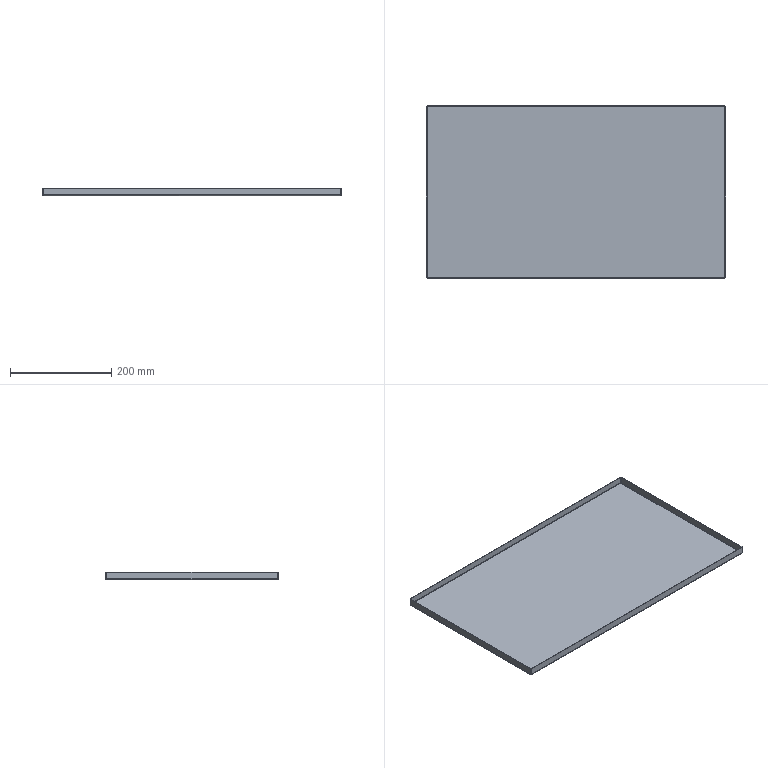Part | NX | features BREP 1 | 1 solid | 38 faces | box 590 x 340 x 15 mm | volume 336698 mm3 | plane 22 | spline 8 | cylinder 8 | commonest cylinder face diameters 1 x4 4 x4
STEP:
#1=CARTESIAN_POINT('',(293.,-168.,-1.5));
#2=VERTEX_POINT('',#1);
#3=CARTESIAN_POINT('',(-293.,-168.,-1.5));
#4=VERTEX_POINT('',#3);
#5=CARTESIAN_POINT('',(293.,-168.,-1.5));
#6=DIRECTION('',(-1.,0.,0.));
#7=VECTOR('',#6,1000.);
#8=LINE('',#5,#7);
#9=EDGE_CURVE('',#2,#4,#8,.T.);
#10=ORIENTED_EDGE('',*,*,#9,.T.);
#11=CARTESIAN_POINT('',(-293.,168.,-1.5));
#12=VERTEX_POINT('',#11);
#13=CARTESIAN_POINT('',(-293.,-168.,-1.5));
#14=DIRECTION('',(0.,1.,0.));
#15=VECTOR('',#14,1000.);
#16=LINE('',#13,#15);
#17=EDGE_CURVE('',#4,#12,#16,.T.);
#18=ORIENTED_EDGE('',*,*,#17,.T.);
#19=CARTESIAN_POINT('',(293.,168.,-1.5));
#20=VERTEX_POINT('',#19);
#21=CARTESIAN_POINT('',(-293.,168.,-1.5));
#22=DIRECTION('',(1.,0.,0.));
#23=VECTOR('',#22,1000.);
#24=LINE('',#21,#23);
#25=EDGE_CURVE('',#12,#20,#24,.T.);
#26=ORIENTED_EDGE('',*,*,#25,.T.);
#27=CARTESIAN_POINT('',(293.,168.,-1.5));
#28=DIRECTION('',(0.,-1.,0.));
#29=VECTOR('',#28,1000.);
#30=LINE('',#27,#29);
#31=EDGE_CURVE('',#20,#2,#30,.T.);
#32=ORIENTED_EDGE('',*,*,#31,.T.);
#33=EDGE_LOOP('',(#10,#18,#26,#32));
#34=FACE_BOUND('',#33,.T.);
#35=CARTESIAN_POINT('',(0.,0.,-1.5));
#36=DIRECTION('',(0.,0.,-1.));
#37=DIRECTION('',(0.,-1.,0.));
#38=AXIS2_PLACEMENT_3D('',#35,#36,#37);
#39=PLANE('',#38);
#40=ADVANCED_FACE('',(#34),#39,.T.);
#41=CARTESIAN_POINT('',(-293.,-168.,0.));
#42=VERTEX_POINT('',#41);
#43=CARTESIAN_POINT('',(-293.,168.,0.));
#44=VERTEX_POINT('',#43);
#45=CARTESIAN_POINT('',(-293.,-168.,0.));
#46=DIRECTION('',(0.,1.,0.));
#47=VECTOR('',#46,1000.);
#48=LINE('',#45,#47);
#49=EDGE_CURVE('',#42,#44,#48,.T.);
#50=ORIENTED_EDGE('',*,*,#49,.F.);
#51=CARTESIAN_POINT('',(293.,-168.,0.));
#52=VERTEX_POINT('',#51);
#53=CARTESIAN_POINT('',(293.,-168.,0.));
#54=DIRECTION('',(-1.,0.,0.));
#55=VECTOR('',#54,1000.);
#56=LINE('',#53,#55);
#57=EDGE_CURVE('',#52,#42,#56,.T.);
#58=ORIENTED_EDGE('',*,*,#57,.F.);
#59=CARTESIAN_POINT('',(293.,168.,0.));
#60=VERTEX_POINT('',#59);
#61=CARTESIAN_POINT('',(293.,168.,0.));
#62=DIRECTION('',(0.,-1.,0.));
#63=VECTOR('',#62,1000.);
#64=LINE('',#61,#63);
#65=EDGE_CURVE('',#60,#52,#64,.T.);
#66=ORIENTED_EDGE('',*,*,#65,.F.);
#67=CARTESIAN_POINT('',(-293.,168.,0.));
#68=DIRECTION('',(1.,0.,0.));
#69=VECTOR('',#68,1000.);
#70=LINE('',#67,#69);
#71=EDGE_CURVE('',#44,#60,#70,.T.);
#72=ORIENTED_EDGE('',*,*,#71,.F.);
#73=EDGE_LOOP('',(#50,#58,#66,#72));
#74=FACE_BOUND('',#73,.T.);
#75=CARTESIAN_POINT('',(0.,0.,0.));
#76=DIRECTION('',(0.,0.,-1.));
#77=DIRECTION('',(0.,-1.,0.));
#78=AXIS2_PLACEMENT_3D('',#75,#76,#77);
#79=PLANE('',#78);
#80=ADVANCED_FACE('',(#74),#79,.F.);
#81=CARTESIAN_POINT('',(292.793,170.,0.5));
#82=VERTEX_POINT('',#81);
#83=CARTESIAN_POINT('',(292.793,168.5,0.5));
#84=VERTEX_POINT('',#83);
#85=CARTESIAN_POINT('',(292.793,168.5,0.5));
#86=DIRECTION('',(0.,-1.,0.));
#87=VECTOR('',#86,1000.);
#88=LINE('',#85,#87);
#89=EDGE_CURVE('',#82,#84,#88,.T.);
#90=ORIENTED_EDGE('',*,*,#89,.T.);
#91=CARTESIAN_POINT('',(293.,168.,0.));
#92=CARTESIAN_POINT('',(292.931,168.262,0.));
#93=CARTESIAN_POINT('',(292.862,168.5,0.2382));
#94=CARTESIAN_POINT('',(292.793,168.5,0.5));
#95=B_SPLINE_CURVE_WITH_KNOTS('',3,(#91,#92,#93,#94),.UNSPECIFIED.,.F.,.F.,(4,4),(0.,1.),.UNSPECIFIED.);
#96=EDGE_CURVE('',#60,#84,#95,.T.);
#97=ORIENTED_EDGE('',*,*,#96,.F.);
#98=CARTESIAN_POINT('',(293.,168.,0.));
#99=DIRECTION('',(0.,0.,-1.));
#100=VECTOR('',#99,1000.);
#101=LINE('',#98,#100);
#102=EDGE_CURVE('',#60,#20,#101,.T.);
#103=ORIENTED_EDGE('',*,*,#102,.T.);
#104=CARTESIAN_POINT('',(292.793,170.,0.5));
#105=CARTESIAN_POINT('',(292.827,170.,-0.0236));
#106=CARTESIAN_POINT('',(292.896,169.567,-1.067));
#107=CARTESIAN_POINT('',(292.965,168.524,-1.5));
#108=CARTESIAN_POINT('',(293.,168.,-1.5));
#109=B_SPLINE_CURVE_WITH_KNOTS('',3,(#104,#105,#106,#107,#108),.UNSPECIFIED.,.F.,.F.,(4,1,4),(0.,0.5,1.),.UNSPECIFIED.);
#110=EDGE_CURVE('',#20,#82,#109,.F.);
#111=ORIENTED_EDGE('',*,*,#110,.T.);
#112=EDGE_LOOP('',(#90,#97,#103,#111));
#113=FACE_BOUND('',#112,.T.);
#114=CARTESIAN_POINT('',(293.,168.,-1.515));
#115=CARTESIAN_POINT('',(292.983,168.264,-1.515));
#116=CARTESIAN_POINT('',(292.965,168.527,-1.463));
#117=CARTESIAN_POINT('',(292.931,169.015,-1.261));
#118=CARTESIAN_POINT('',(292.914,169.238,-1.111));
#119=CARTESIAN_POINT('',(292.879,169.611,-0.7383));
#120=CARTESIAN_POINT('',(292.862,169.761,-0.5148));
#121=CARTESIAN_POINT('',(292.827,169.963,-0.02742));
#122=CARTESIAN_POINT('',(292.81,170.015,0.2362));
#123=CARTESIAN_POINT('',(292.793,170.015,0.5));
#124=CARTESIAN_POINT('',(293.,168.,-1.5));
#125=CARTESIAN_POINT('',(292.983,168.262,-1.5));
#126=CARTESIAN_POINT('',(292.965,168.523,-1.448));
#127=CARTESIAN_POINT('',(292.931,169.007,-1.248));
#128=CARTESIAN_POINT('',(292.914,169.229,-1.099));
#129=CARTESIAN_POINT('',(292.879,169.599,-0.7291));
#130=CARTESIAN_POINT('',(292.862,169.748,-0.5072));
#131=CARTESIAN_POINT('',(292.827,169.948,-0.0235));
#132=CARTESIAN_POINT('',(292.81,170.,0.2382));
#133=CARTESIAN_POINT('',(292.793,170.,0.5));
#134=CARTESIAN_POINT('',(293.,168.,0.));
#135=CARTESIAN_POINT('',(292.983,168.065,0.));
#136=CARTESIAN_POINT('',(292.965,168.131,0.01301));
#137=CARTESIAN_POINT('',(292.931,168.252,0.06311));
#138=CARTESIAN_POINT('',(292.914,168.307,0.1002));
#139=CARTESIAN_POINT('',(292.879,168.4,0.1927));
#140=CARTESIAN_POINT('',(292.862,168.437,0.2482));
#141=CARTESIAN_POINT('',(292.827,168.487,0.3691));
#142=CARTESIAN_POINT('',(292.81,168.5,0.4345));
#143=CARTESIAN_POINT('',(292.793,168.5,0.5));
#144=CARTESIAN_POINT('',(293.,168.,0.01515));
#145=CARTESIAN_POINT('',(292.983,168.063,0.01515));
#146=CARTESIAN_POINT('',(292.965,168.127,0.02777));
#147=CARTESIAN_POINT('',(292.931,168.244,0.07634));
#148=CARTESIAN_POINT('',(292.914,168.298,0.1123));
#149=CARTESIAN_POINT('',(292.879,168.388,0.202));
#150=CARTESIAN_POINT('',(292.862,168.424,0.2558));
#151=CARTESIAN_POINT('',(292.827,168.472,0.3731));
#152=CARTESIAN_POINT('',(292.81,168.485,0.4365));
#153=CARTESIAN_POINT('',(292.793,168.485,0.5));
#154=B_SPLINE_SURFACE_WITH_KNOTS('',1,3,((#114,#115,#116,#117,#118,#119,#120,#121,#122,#123),(#124,#125,#126,#127,#128,#129,#130,#131,#132,#133),(#134,#135,#136,#137,#138,#139,#140,#141,#142,#143),(#144,#145,#146,#147,#148,#149,#150,#151,#152,#153)),.RULED_SURF.,.F.,.F.,.F.,(2,1,1,2),(4,2,2,2,4),(-0.01,0.,1.,1.01),(0.,0.25,0.5,0.75,1.),.UNSPECIFIED.);
#155=ADVANCED_FACE('',(#113),#154,.F.);
#156=CARTESIAN_POINT('',(-292.793,168.5,0.5));
#157=VERTEX_POINT('',#156);
#158=CARTESIAN_POINT('',(-292.793,168.5,0.5));
#159=CARTESIAN_POINT('',(-292.862,168.5,0.2382));
#160=CARTESIAN_POINT('',(-292.931,168.262,0.));
#161=CARTESIAN_POINT('',(-293.,168.,0.));
#162=B_SPLINE_CURVE_WITH_KNOTS('',3,(#158,#159,#160,#161),.UNSPECIFIED.,.F.,.F.,(4,4),(0.,1.),.UNSPECIFIED.);
#163=EDGE_CURVE('',#157,#44,#162,.T.);
#164=ORIENTED_EDGE('',*,*,#163,.F.);
#165=CARTESIAN_POINT('',(-292.793,170.,0.5));
#166=VERTEX_POINT('',#165);
#167=CARTESIAN_POINT('',(-292.793,168.5,0.5));
#168=DIRECTION('',(0.,-1.,0.));
#169=VECTOR('',#168,1000.);
#170=LINE('',#167,#169);
#171=EDGE_CURVE('',#166,#157,#170,.T.);
#172=ORIENTED_EDGE('',*,*,#171,.F.);
#173=CARTESIAN_POINT('',(-293.,168.,-1.5));
#174=CARTESIAN_POINT('',(-292.965,168.524,-1.5));
#175=CARTESIAN_POINT('',(-292.896,169.567,-1.067));
#176=CARTESIAN_POINT('',(-292.827,170.,-0.0236));
#177=CARTESIAN_POINT('',(-292.793,170.,0.5));
#178=B_SPLINE_CURVE_WITH_KNOTS('',3,(#173,#174,#175,#176,#177),.UNSPECIFIED.,.F.,.F.,(4,1,4),(0.,0.5,1.),.UNSPECIFIED.);
#179=EDGE_CURVE('',#166,#12,#178,.F.);
#180=ORIENTED_EDGE('',*,*,#179,.T.);
#181=CARTESIAN_POINT('',(-293.,168.,0.));
#182=DIRECTION('',(0.,0.,-1.));
#183=VECTOR('',#182,1000.);
#184=LINE('',#181,#183);
#185=EDGE_CURVE('',#44,#12,#184,.T.);
#186=ORIENTED_EDGE('',*,*,#185,.F.);
#187=EDGE_LOOP('',(#164,#172,#180,#186));
#188=FACE_BOUND('',#187,.T.);
#189=CARTESIAN_POINT('',(-292.793,170.015,0.5));
#190=CARTESIAN_POINT('',(-292.81,170.015,0.2362));
#191=CARTESIAN_POINT('',(-292.827,169.963,-0.02742));
#192=CARTESIAN_POINT('',(-292.862,169.761,-0.5148));
#193=CARTESIAN_POINT('',(-292.879,169.611,-0.7383));
#194=CARTESIAN_POINT('',(-292.914,169.238,-1.111));
#195=CARTESIAN_POINT('',(-292.931,169.015,-1.261));
#196=CARTESIAN_POINT('',(-292.965,168.527,-1.463));
#197=CARTESIAN_POINT('',(-292.983,168.264,-1.515));
#198=CARTESIAN_POINT('',(-293.,168.,-1.515));
#199=CARTESIAN_POINT('',(-292.793,170.,0.5));
#200=CARTESIAN_POINT('',(-292.81,170.,0.2382));
#201=CARTESIAN_POINT('',(-292.827,169.948,-0.0235));
#202=CARTESIAN_POINT('',(-292.862,169.748,-0.5072));
#203=CARTESIAN_POINT('',(-292.879,169.599,-0.7291));
#204=CARTESIAN_POINT('',(-292.914,169.229,-1.099));
#205=CARTESIAN_POINT('',(-292.931,169.007,-1.248));
#206=CARTESIAN_POINT('',(-292.965,168.523,-1.448));
#207=CARTESIAN_POINT('',(-292.983,168.262,-1.5));
#208=CARTESIAN_POINT('',(-293.,168.,-1.5));
#209=CARTESIAN_POINT('',(-292.793,168.5,0.5));
#210=CARTESIAN_POINT('',(-292.81,168.5,0.4345));
#211=CARTESIAN_POINT('',(-292.827,168.487,0.3691));
#212=CARTESIAN_POINT('',(-292.862,168.437,0.2482));
#213=CARTESIAN_POINT('',(-292.879,168.4,0.1927));
#214=CARTESIAN_POINT('',(-292.914,168.307,0.1002));
#215=CARTESIAN_POINT('',(-292.931,168.252,0.06311));
#216=CARTESIAN_POINT('',(-292.965,168.131,0.01301));
#217=CARTESIAN_POINT('',(-292.983,168.065,0.));
#218=CARTESIAN_POINT('',(-293.,168.,0.));
#219=CARTESIAN_POINT('',(-292.793,168.485,0.5));
#220=CARTESIAN_POINT('',(-292.81,168.485,0.4365));
#221=CARTESIAN_POINT('',(-292.827,168.472,0.3731));
#222=CARTESIAN_POINT('',(-292.862,168.424,0.2558));
#223=CARTESIAN_POINT('',(-292.879,168.388,0.202));
#224=CARTESIAN_POINT('',(-292.914,168.298,0.1123));
#225=CARTESIAN_POINT('',(-292.931,168.244,0.07634));
#226=CARTESIAN_POINT('',(-292.965,168.127,0.02777));
#227=CARTESIAN_POINT('',(-292.983,168.063,0.01515));
#228=CARTESIAN_POINT('',(-293.,168.,0.01515));
#229=B_SPLINE_SURFACE_WITH_KNOTS('',1,3,((#189,#190,#191,#192,#193,#194,#195,#196,#197,#198),(#199,#200,#201,#202,#203,#204,#205,#206,#207,#208),(#209,#210,#211,#212,#213,#214,#215,#216,#217,#218),(#219,#220,#221,#222,#223,#224,#225,#226,#227,#228)),.RULED_SURF.,.F.,.F.,.F.,(2,1,1,2),(4,2,2,2,4),(-0.01,0.,1.,1.01),(0.,0.25,0.5,0.75,1.),.UNSPECIFIED.);
#230=ADVANCED_FACE('',(#188),#229,.F.);
#231=ORIENTED_EDGE('',*,*,#25,.F.);
#232=ORIENTED_EDGE('',*,*,#179,.F.);
#233=CARTESIAN_POINT('',(0.,170.,0.5));
#234=DIRECTION('',(-1.,0.,0.));
#235=VECTOR('',#234,1000.);
#236=LINE('',#233,#235);
#237=EDGE_CURVE('',#82,#166,#236,.T.);
#238=ORIENTED_EDGE('',*,*,#237,.F.);
#239=ORIENTED_EDGE('',*,*,#110,.F.);
#240=EDGE_LOOP('',(#231,#232,#238,#239));
#241=FACE_BOUND('',#240,.T.);
#242=CARTESIAN_POINT('',(-293.,168.,0.5));
#243=DIRECTION('',(-1.,0.,0.));
#244=DIRECTION('',(0.,1.,0.));
#245=AXIS2_PLACEMENT_3D('',#242,#243,#244);
#246=CYLINDRICAL_SURFACE('',#245,2.);
#247=ADVANCED_FACE('',(#241),#246,.T.);
#248=ORIENTED_EDGE('',*,*,#71,.T.);
#249=ORIENTED_EDGE('',*,*,#96,.T.);
#250=CARTESIAN_POINT('',(295.,168.5,0.5));
#251=DIRECTION('',(-1.,0.,0.));
#252=VECTOR('',#251,1000.);
#253=LINE('',#250,#252);
#254=EDGE_CURVE('',#84,#157,#253,.T.);
#255=ORIENTED_EDGE('',*,*,#254,.T.);
#256=ORIENTED_EDGE('',*,*,#163,.T.);
#257=EDGE_LOOP('',(#248,#249,#255,#256));
#258=FACE_BOUND('',#257,.T.);
#259=CARTESIAN_POINT('',(-293.,168.,0.5));
#260=DIRECTION('',(-1.,0.,0.));
#261=DIRECTION('',(0.,1.,0.));
#262=AXIS2_PLACEMENT_3D('',#259,#260,#261);
#263=CYLINDRICAL_SURFACE('',#262,0.5);
#264=ADVANCED_FACE('',(#258),#263,.F.);
#265=CARTESIAN_POINT('',(292.793,168.5,13.5));
#266=VERTEX_POINT('',#265);
#267=CARTESIAN_POINT('',(292.793,170.,13.5));
#268=VERTEX_POINT('',#267);
#269=CARTESIAN_POINT('',(292.793,170.,13.5));
#270=DIRECTION('',(0.,1.,0.));
#271=VECTOR('',#270,1000.);
#272=LINE('',#269,#271);
#273=EDGE_CURVE('',#266,#268,#272,.T.);
#274=ORIENTED_EDGE('',*,*,#273,.F.);
#275=CARTESIAN_POINT('',(292.793,168.5,0.));
#276=DIRECTION('',(0.,0.,1.));
#277=VECTOR('',#276,1000.);
#278=LINE('',#275,#277);
#279=EDGE_CURVE('',#84,#266,#278,.T.);
#280=ORIENTED_EDGE('',*,*,#279,.F.);
#281=ORIENTED_EDGE('',*,*,#89,.F.);
#282=CARTESIAN_POINT('',(292.793,170.,0.));
#283=DIRECTION('',(0.,0.,-1.));
#284=VECTOR('',#283,1000.);
#285=LINE('',#282,#284);
#286=EDGE_CURVE('',#268,#82,#285,.T.);
#287=ORIENTED_EDGE('',*,*,#286,.F.);
#288=EDGE_LOOP('',(#274,#280,#281,#287));
#289=FACE_BOUND('',#288,.T.);
#290=CARTESIAN_POINT('',(292.793,168.5,0.));
#291=DIRECTION('',(1.,0.,0.));
#292=DIRECTION('',(0.,1.,0.));
#293=AXIS2_PLACEMENT_3D('',#290,#291,#292);
#294=PLANE('',#293);
#295=ADVANCED_FACE('',(#289),#294,.T.);
#296=CARTESIAN_POINT('',(-292.793,170.,13.5));
#297=VERTEX_POINT('',#296);
#298=CARTESIAN_POINT('',(-292.793,170.,0.));
#299=DIRECTION('',(0.,0.,-1.));
#300=VECTOR('',#299,1000.);
#301=LINE('',#298,#300);
#302=EDGE_CURVE('',#297,#166,#301,.T.);
#303=ORIENTED_EDGE('',*,*,#302,.F.);
#304=CARTESIAN_POINT('',(-295.,170.,13.5));
#305=DIRECTION('',(-1.,0.,0.));
#306=VECTOR('',#305,1000.);
#307=LINE('',#304,#306);
#308=EDGE_CURVE('',#268,#297,#307,.T.);
#309=ORIENTED_EDGE('',*,*,#308,.F.);
#310=ORIENTED_EDGE('',*,*,#286,.T.);
#311=ORIENTED_EDGE('',*,*,#237,.T.);
#312=EDGE_LOOP('',(#303,#309,#310,#311));
#313=FACE_BOUND('',#312,.T.);
#314=CARTESIAN_POINT('',(0.,170.,0.));
#315=DIRECTION('',(0.,1.,0.));
#316=DIRECTION('',(0.,0.,-1.));
#317=AXIS2_PLACEMENT_3D('',#314,#315,#316);
#318=PLANE('',#317);
#319=ADVANCED_FACE('',(#313),#318,.T.);
#320=CARTESIAN_POINT('',(-292.793,168.5,13.5));
#321=VERTEX_POINT('',#320);
#322=CARTESIAN_POINT('',(0.,168.5,13.5));
#323=DIRECTION('',(-1.,0.,0.));
#324=VECTOR('',#323,1000.);
#325=LINE('',#322,#324);
#326=EDGE_CURVE('',#266,#321,#325,.T.);
#327=ORIENTED_EDGE('',*,*,#326,.T.);
#328=CARTESIAN_POINT('',(-292.793,168.5,0.));
#329=DIRECTION('',(0.,0.,1.));
#330=VECTOR('',#329,1000.);
#331=LINE('',#328,#330);
#332=EDGE_CURVE('',#157,#321,#331,.T.);
#333=ORIENTED_EDGE('',*,*,#332,.F.);
#334=ORIENTED_EDGE('',*,*,#254,.F.);
#335=ORIENTED_EDGE('',*,*,#279,.T.);
#336=EDGE_LOOP('',(#327,#333,#334,#335));
#337=FACE_BOUND('',#336,.T.);
#338=CARTESIAN_POINT('',(0.,168.5,0.));
#339=DIRECTION('',(0.,1.,0.));
#340=DIRECTION('',(0.,0.,-1.));
#341=AXIS2_PLACEMENT_3D('',#338,#339,#340);
#342=PLANE('',#341);
#343=ADVANCED_FACE('',(#337),#342,.F.);
#344=CARTESIAN_POINT('',(-292.793,168.5,13.5));
#345=DIRECTION('',(0.,1.,0.));
#346=VECTOR('',#345,1000.);
#347=LINE('',#344,#346);
#348=EDGE_CURVE('',#321,#297,#347,.T.);
#349=ORIENTED_EDGE('',*,*,#348,.F.);
#350=ORIENTED_EDGE('',*,*,#326,.F.);
#351=ORIENTED_EDGE('',*,*,#273,.T.);
#352=ORIENTED_EDGE('',*,*,#308,.T.);
#353=EDGE_LOOP('',(#349,#350,#351,#352));
#354=FACE_BOUND('',#353,.T.);
#355=CARTESIAN_POINT('',(-295.,170.,13.5));
#356=DIRECTION('',(0.,0.,1.));
#357=DIRECTION('',(0.,-1.,0.));
#358=AXIS2_PLACEMENT_3D('',#355,#356,#357);
#359=PLANE('',#358);
#360=ADVANCED_FACE('',(#354),#359,.T.);
#361=ORIENTED_EDGE('',*,*,#332,.T.);
#362=ORIENTED_EDGE('',*,*,#348,.T.);
#363=ORIENTED_EDGE('',*,*,#302,.T.);
#364=ORIENTED_EDGE('',*,*,#171,.T.);
#365=EDGE_LOOP('',(#361,#362,#363,#364));
#366=FACE_BOUND('',#365,.T.);
#367=CARTESIAN_POINT('',(-292.793,168.5,0.));
#368=DIRECTION('',(1.,0.,0.));
#369=DIRECTION('',(0.,1.,0.));
#370=AXIS2_PLACEMENT_3D('',#367,#368,#369);
#371=PLANE('',#370);
#372=ADVANCED_FACE('',(#366),#371,.F.);
#373=CARTESIAN_POINT('',(295.,-167.793,0.5));
#374=VERTEX_POINT('',#373);
#375=CARTESIAN_POINT('',(293.5,-167.793,0.5));
#376=VERTEX_POINT('',#375);
#377=CARTESIAN_POINT('',(293.5,-167.793,0.5));
#378=DIRECTION('',(-1.,0.,0.));
#379=VECTOR('',#378,1000.);
#380=LINE('',#377,#379);
#381=EDGE_CURVE('',#374,#376,#380,.T.);
#382=ORIENTED_EDGE('',*,*,#381,.T.);
#383=CARTESIAN_POINT('',(293.,-168.,0.));
#384=CARTESIAN_POINT('',(293.262,-167.931,0.));
#385=CARTESIAN_POINT('',(293.5,-167.862,0.2382));
#386=CARTESIAN_POINT('',(293.5,-167.793,0.5));
#387=B_SPLINE_CURVE_WITH_KNOTS('',3,(#383,#384,#385,#386),.UNSPECIFIED.,.F.,.F.,(4,4),(0.,1.),.UNSPECIFIED.);
#388=EDGE_CURVE('',#52,#376,#387,.T.);
#389=ORIENTED_EDGE('',*,*,#388,.F.);
#390=CARTESIAN_POINT('',(293.,-168.,0.));
#391=DIRECTION('',(0.,0.,-1.));
#392=VECTOR('',#391,1000.);
#393=LINE('',#390,#392);
#394=EDGE_CURVE('',#52,#2,#393,.T.);
#395=ORIENTED_EDGE('',*,*,#394,.T.);
#396=CARTESIAN_POINT('',(295.,-167.793,0.5));
#397=CARTESIAN_POINT('',(295.,-167.827,-0.0236));
#398=CARTESIAN_POINT('',(294.567,-167.896,-1.067));
#399=CARTESIAN_POINT('',(293.524,-167.965,-1.5));
#400=CARTESIAN_POINT('',(293.,-168.,-1.5));
#401=B_SPLINE_CURVE_WITH_KNOTS('',3,(#396,#397,#398,#399,#400),.UNSPECIFIED.,.F.,.F.,(4,1,4),(0.,0.5,1.),.UNSPECIFIED.);
#402=EDGE_CURVE('',#2,#374,#401,.F.);
#403=ORIENTED_EDGE('',*,*,#402,.T.);
#404=EDGE_LOOP('',(#382,#389,#395,#403));
#405=FACE_BOUND('',#404,.T.);
#406=CARTESIAN_POINT('',(293.,-168.,-1.515));
#407=CARTESIAN_POINT('',(293.264,-167.983,-1.515));
#408=CARTESIAN_POINT('',(293.527,-167.965,-1.463));
#409=CARTESIAN_POINT('',(294.015,-167.931,-1.261));
#410=CARTESIAN_POINT('',(294.238,-167.914,-1.111));
#411=CARTESIAN_POINT('',(294.611,-167.879,-0.7383));
#412=CARTESIAN_POINT('',(294.761,-167.862,-0.5148));
#413=CARTESIAN_POINT('',(294.963,-167.827,-0.02742));
#414=CARTESIAN_POINT('',(295.015,-167.81,0.2362));
#415=CARTESIAN_POINT('',(295.015,-167.793,0.5));
#416=CARTESIAN_POINT('',(293.,-168.,-1.5));
#417=CARTESIAN_POINT('',(293.262,-167.983,-1.5));
#418=CARTESIAN_POINT('',(293.523,-167.965,-1.448));
#419=CARTESIAN_POINT('',(294.007,-167.931,-1.248));
#420=CARTESIAN_POINT('',(294.229,-167.914,-1.099));
#421=CARTESIAN_POINT('',(294.599,-167.879,-0.7291));
#422=CARTESIAN_POINT('',(294.748,-167.862,-0.5072));
#423=CARTESIAN_POINT('',(294.948,-167.827,-0.0235));
#424=CARTESIAN_POINT('',(295.,-167.81,0.2382));
#425=CARTESIAN_POINT('',(295.,-167.793,0.5));
#426=CARTESIAN_POINT('',(293.,-168.,0.));
#427=CARTESIAN_POINT('',(293.065,-167.983,0.));
#428=CARTESIAN_POINT('',(293.131,-167.965,0.01301));
#429=CARTESIAN_POINT('',(293.252,-167.931,0.06311));
#430=CARTESIAN_POINT('',(293.307,-167.914,0.1002));
#431=CARTESIAN_POINT('',(293.4,-167.879,0.1927));
#432=CARTESIAN_POINT('',(293.437,-167.862,0.2482));
#433=CARTESIAN_POINT('',(293.487,-167.827,0.3691));
#434=CARTESIAN_POINT('',(293.5,-167.81,0.4345));
#435=CARTESIAN_POINT('',(293.5,-167.793,0.5));
#436=CARTESIAN_POINT('',(293.,-168.,0.01515));
#437=CARTESIAN_POINT('',(293.063,-167.983,0.01515));
#438=CARTESIAN_POINT('',(293.127,-167.965,0.02777));
#439=CARTESIAN_POINT('',(293.244,-167.931,0.07634));
#440=CARTESIAN_POINT('',(293.298,-167.914,0.1123));
#441=CARTESIAN_POINT('',(293.388,-167.879,0.202));
#442=CARTESIAN_POINT('',(293.424,-167.862,0.2558));
#443=CARTESIAN_POINT('',(293.472,-167.827,0.3731));
#444=CARTESIAN_POINT('',(293.485,-167.81,0.4365));
#445=CARTESIAN_POINT('',(293.485,-167.793,0.5));
#446=B_SPLINE_SURFACE_WITH_KNOTS('',1,3,((#406,#407,#408,#409,#410,#411,#412,#413,#414,#415),(#416,#417,#418,#419,#420,#421,#422,#423,#424,#425),(#426,#427,#428,#429,#430,#431,#432,#433,#434,#435),(#436,#437,#438,#439,#440,#441,#442,#443,#444,#445)),.RULED_SURF.,.F.,.F.,.F.,(2,1,1,2),(4,2,2,2,4),(-0.01,0.,1.,1.01),(0.,0.25,0.5,0.75,1.),.UNSPECIFIED.);
#447=ADVANCED_FACE('',(#405),#446,.F.);
#448=CARTESIAN_POINT('',(293.5,167.793,0.5));
#449=VERTEX_POINT('',#448);
#450=CARTESIAN_POINT('',(293.5,167.793,0.5));
#451=CARTESIAN_POINT('',(293.5,167.862,0.2382));
#452=CARTESIAN_POINT('',(293.262,167.931,0.));
#453=CARTESIAN_POINT('',(293.,168.,0.));
#454=B_SPLINE_CURVE_WITH_KNOTS('',3,(#450,#451,#452,#453),.UNSPECIFIED.,.F.,.F.,(4,4),(0.,1.),.UNSPECIFIED.);
#455=EDGE_CURVE('',#449,#60,#454,.T.);
#456=ORIENTED_EDGE('',*,*,#455,.F.);
#457=CARTESIAN_POINT('',(295.,167.793,0.5));
#458=VERTEX_POINT('',#457);
#459=CARTESIAN_POINT('',(293.5,167.793,0.5));
#460=DIRECTION('',(-1.,0.,0.));
#461=VECTOR('',#460,1000.);
#462=LINE('',#459,#461);
#463=EDGE_CURVE('',#458,#449,#462,.T.);
#464=ORIENTED_EDGE('',*,*,#463,.F.);
#465=CARTESIAN_POINT('',(293.,168.,-1.5));
#466=CARTESIAN_POINT('',(293.524,167.965,-1.5));
#467=CARTESIAN_POINT('',(294.567,167.896,-1.067));
#468=CARTESIAN_POINT('',(295.,167.827,-0.0236));
#469=CARTESIAN_POINT('',(295.,167.793,0.5));
#470=B_SPLINE_CURVE_WITH_KNOTS('',3,(#465,#466,#467,#468,#469),.UNSPECIFIED.,.F.,.F.,(4,1,4),(0.,0.5,1.),.UNSPECIFIED.);
#471=EDGE_CURVE('',#458,#20,#470,.F.);
#472=ORIENTED_EDGE('',*,*,#471,.T.);
#473=ORIENTED_EDGE('',*,*,#102,.F.);
#474=EDGE_LOOP('',(#456,#464,#472,#473));
#475=FACE_BOUND('',#474,.T.);
#476=CARTESIAN_POINT('',(295.015,167.793,0.5));
#477=CARTESIAN_POINT('',(295.015,167.81,0.2362));
#478=CARTESIAN_POINT('',(294.963,167.827,-0.02742));
#479=CARTESIAN_POINT('',(294.761,167.862,-0.5148));
#480=CARTESIAN_POINT('',(294.611,167.879,-0.7383));
#481=CARTESIAN_POINT('',(294.238,167.914,-1.111));
#482=CARTESIAN_POINT('',(294.015,167.931,-1.261));
#483=CARTESIAN_POINT('',(293.527,167.965,-1.463));
#484=CARTESIAN_POINT('',(293.264,167.983,-1.515));
#485=CARTESIAN_POINT('',(293.,168.,-1.515));
#486=CARTESIAN_POINT('',(295.,167.793,0.5));
#487=CARTESIAN_POINT('',(295.,167.81,0.2382));
#488=CARTESIAN_POINT('',(294.948,167.827,-0.0235));
#489=CARTESIAN_POINT('',(294.748,167.862,-0.5072));
#490=CARTESIAN_POINT('',(294.599,167.879,-0.7291));
#491=CARTESIAN_POINT('',(294.229,167.914,-1.099));
#492=CARTESIAN_POINT('',(294.007,167.931,-1.248));
#493=CARTESIAN_POINT('',(293.523,167.965,-1.448));
#494=CARTESIAN_POINT('',(293.262,167.983,-1.5));
#495=CARTESIAN_POINT('',(293.,168.,-1.5));
#496=CARTESIAN_POINT('',(293.5,167.793,0.5));
#497=CARTESIAN_POINT('',(293.5,167.81,0.4345));
#498=CARTESIAN_POINT('',(293.487,167.827,0.3691));
#499=CARTESIAN_POINT('',(293.437,167.862,0.2482));
#500=CARTESIAN_POINT('',(293.4,167.879,0.1927));
#501=CARTESIAN_POINT('',(293.307,167.914,0.1002));
#502=CARTESIAN_POINT('',(293.252,167.931,0.06311));
#503=CARTESIAN_POINT('',(293.131,167.965,0.01301));
#504=CARTESIAN_POINT('',(293.065,167.983,0.));
#505=CARTESIAN_POINT('',(293.,168.,0.));
#506=CARTESIAN_POINT('',(293.485,167.793,0.5));
#507=CARTESIAN_POINT('',(293.485,167.81,0.4365));
#508=CARTESIAN_POINT('',(293.472,167.827,0.3731));
#509=CARTESIAN_POINT('',(293.424,167.862,0.2558));
#510=CARTESIAN_POINT('',(293.388,167.879,0.202));
#511=CARTESIAN_POINT('',(293.298,167.914,0.1123));
#512=CARTESIAN_POINT('',(293.244,167.931,0.07634));
#513=CARTESIAN_POINT('',(293.127,167.965,0.02777));
#514=CARTESIAN_POINT('',(293.063,167.983,0.01515));
#515=CARTESIAN_POINT('',(293.,168.,0.01515));
#516=B_SPLINE_SURFACE_WITH_KNOTS('',1,3,((#476,#477,#478,#479,#480,#481,#482,#483,#484,#485),(#486,#487,#488,#489,#490,#491,#492,#493,#494,#495),(#496,#497,#498,#499,#500,#501,#502,#503,#504,#505),(#506,#507,#508,#509,#510,#511,#512,#513,#514,#515)),.RULED_SURF.,.F.,.F.,.F.,(2,1,1,2),(4,2,2,2,4),(-0.01,0.,1.,1.01),(0.,0.25,0.5,0.75,1.),.UNSPECIFIED.);
#517=ADVANCED_FACE('',(#475),#516,.F.);
#518=ORIENTED_EDGE('',*,*,#31,.F.);
#519=ORIENTED_EDGE('',*,*,#471,.F.);
#520=CARTESIAN_POINT('',(295.,-170.,0.5));
#521=DIRECTION('',(0.,-1.,0.));
#522=VECTOR('',#521,1000.);
#523=LINE('',#520,#522);
#524=EDGE_CURVE('',#458,#374,#523,.T.);
#525=ORIENTED_EDGE('',*,*,#524,.T.);
#526=ORIENTED_EDGE('',*,*,#402,.F.);
#527=EDGE_LOOP('',(#518,#519,#525,#526));
#528=FACE_BOUND('',#527,.T.);
#529=CARTESIAN_POINT('',(293.,168.,0.5));
#530=DIRECTION('',(0.,1.,0.));
#531=DIRECTION('',(1.,0.,0.));
#532=AXIS2_PLACEMENT_3D('',#529,#530,#531);
#533=CYLINDRICAL_SURFACE('',#532,2.);
#534=ADVANCED_FACE('',(#528),#533,.T.);
#535=ORIENTED_EDGE('',*,*,#65,.T.);
#536=ORIENTED_EDGE('',*,*,#388,.T.);
#537=CARTESIAN_POINT('',(293.5,-170.,0.5));
#538=DIRECTION('',(0.,1.,0.));
#539=VECTOR('',#538,1000.);
#540=LINE('',#537,#539);
#541=EDGE_CURVE('',#376,#449,#540,.T.);
#542=ORIENTED_EDGE('',*,*,#541,.T.);
#543=ORIENTED_EDGE('',*,*,#455,.T.);
#544=EDGE_LOOP('',(#535,#536,#542,#543));
#545=FACE_BOUND('',#544,.T.);
#546=CARTESIAN_POINT('',(293.,168.,0.5));
#547=DIRECTION('',(0.,1.,0.));
#548=DIRECTION('',(1.,0.,0.));
#549=AXIS2_PLACEMENT_3D('',#546,#547,#548);
#550=CYLINDRICAL_SURFACE('',#549,0.5);
#551=ADVANCED_FACE('',(#545),#550,.F.);
#552=CARTESIAN_POINT('',(293.5,-167.793,13.5));
#553=VERTEX_POINT('',#552);
#554=CARTESIAN_POINT('',(295.,-167.793,13.5));
#555=VERTEX_POINT('',#554);
#556=CARTESIAN_POINT('',(295.,-167.793,13.5));
#557=DIRECTION('',(1.,0.,0.));
#558=VECTOR('',#557,1000.);
#559=LINE('',#556,#558);
#560=EDGE_CURVE('',#553,#555,#559,.T.);
#561=ORIENTED_EDGE('',*,*,#560,.F.);
#562=CARTESIAN_POINT('',(293.5,-167.793,0.));
#563=DIRECTION('',(0.,0.,1.));
#564=VECTOR('',#563,1000.);
#565=LINE('',#562,#564);
#566=EDGE_CURVE('',#376,#553,#565,.T.);
#567=ORIENTED_EDGE('',*,*,#566,.F.);
#568=ORIENTED_EDGE('',*,*,#381,.F.);
#569=CARTESIAN_POINT('',(295.,-167.793,0.));
#570=DIRECTION('',(0.,0.,1.));
#571=VECTOR('',#570,1000.);
#572=LINE('',#569,#571);
#573=EDGE_CURVE('',#374,#555,#572,.T.);
#574=ORIENTED_EDGE('',*,*,#573,.T.);
#575=EDGE_LOOP('',(#561,#567,#568,#574));
#576=FACE_BOUND('',#575,.T.);
#577=CARTESIAN_POINT('',(293.5,-167.793,0.));
#578=DIRECTION('',(0.,-1.,0.));
#579=DIRECTION('',(0.,0.,-1.));
#580=AXIS2_PLACEMENT_3D('',#577,#578,#579);
#581=PLANE('',#580);
#582=ADVANCED_FACE('',(#576),#581,.T.);
#583=ORIENTED_EDGE('',*,*,#524,.F.);
#584=CARTESIAN_POINT('',(295.,167.793,13.5));
#585=VERTEX_POINT('',#584);
#586=CARTESIAN_POINT('',(295.,167.793,0.));
#587=DIRECTION('',(0.,0.,1.));
#588=VECTOR('',#587,1000.);
#589=LINE('',#586,#588);
#590=EDGE_CURVE('',#458,#585,#589,.T.);
#591=ORIENTED_EDGE('',*,*,#590,.T.);
#592=CARTESIAN_POINT('',(295.,-170.,13.5));
#593=DIRECTION('',(0.,1.,0.));
#594=VECTOR('',#593,1000.);
#595=LINE('',#592,#594);
#596=EDGE_CURVE('',#555,#585,#595,.T.);
#597=ORIENTED_EDGE('',*,*,#596,.F.);
#598=ORIENTED_EDGE('',*,*,#573,.F.);
#599=EDGE_LOOP('',(#583,#591,#597,#598));
#600=FACE_BOUND('',#599,.T.);
#601=CARTESIAN_POINT('',(295.,0.,0.));
#602=DIRECTION('',(-1.,0.,0.));
#603=DIRECTION('',(0.,1.,0.));
#604=AXIS2_PLACEMENT_3D('',#601,#602,#603);
#605=PLANE('',#604);
#606=ADVANCED_FACE('',(#600),#605,.F.);
#607=CARTESIAN_POINT('',(293.5,167.793,13.5));
#608=VERTEX_POINT('',#607);
#609=CARTESIAN_POINT('',(293.5,167.793,0.));
#610=DIRECTION('',(0.,0.,1.));
#611=VECTOR('',#610,1000.);
#612=LINE('',#609,#611);
#613=EDGE_CURVE('',#449,#608,#612,.T.);
#614=ORIENTED_EDGE('',*,*,#613,.F.);
#615=ORIENTED_EDGE('',*,*,#541,.F.);
#616=ORIENTED_EDGE('',*,*,#566,.T.);
#617=CARTESIAN_POINT('',(293.5,0.,13.5));
#618=DIRECTION('',(0.,1.,0.));
#619=VECTOR('',#618,1000.);
#620=LINE('',#617,#619);
#621=EDGE_CURVE('',#553,#608,#620,.T.);
#622=ORIENTED_EDGE('',*,*,#621,.T.);
#623=EDGE_LOOP('',(#614,#615,#616,#622));
#624=FACE_BOUND('',#623,.T.);
#625=CARTESIAN_POINT('',(293.5,0.,0.));
#626=DIRECTION('',(-1.,0.,0.));
#627=DIRECTION('',(0.,1.,0.));
#628=AXIS2_PLACEMENT_3D('',#625,#626,#627);
#629=PLANE('',#628);
#630=ADVANCED_FACE('',(#624),#629,.T.);
#631=CARTESIAN_POINT('',(293.5,167.793,13.5));
#632=DIRECTION('',(1.,0.,0.));
#633=VECTOR('',#632,1000.);
#634=LINE('',#631,#633);
#635=EDGE_CURVE('',#608,#585,#634,.T.);
#636=ORIENTED_EDGE('',*,*,#635,.F.);
#637=ORIENTED_EDGE('',*,*,#621,.F.);
#638=ORIENTED_EDGE('',*,*,#560,.T.);
#639=ORIENTED_EDGE('',*,*,#596,.T.);
#640=EDGE_LOOP('',(#636,#637,#638,#639));
#641=FACE_BOUND('',#640,.T.);
#642=CARTESIAN_POINT('',(295.,-170.,13.5));
#643=DIRECTION('',(0.,0.,1.));
#644=DIRECTION('',(1.,0.,0.));
#645=AXIS2_PLACEMENT_3D('',#642,#643,#644);
#646=PLANE('',#645);
#647=ADVANCED_FACE('',(#641),#646,.T.);
#648=ORIENTED_EDGE('',*,*,#613,.T.);
#649=ORIENTED_EDGE('',*,*,#635,.T.);
#650=ORIENTED_EDGE('',*,*,#590,.F.);
#651=ORIENTED_EDGE('',*,*,#463,.T.);
#652=EDGE_LOOP('',(#648,#649,#650,#651));
#653=FACE_BOUND('',#652,.T.);
#654=CARTESIAN_POINT('',(293.5,167.793,0.));
#655=DIRECTION('',(0.,-1.,0.));
#656=DIRECTION('',(0.,0.,-1.));
#657=AXIS2_PLACEMENT_3D('',#654,#655,#656);
#658=PLANE('',#657);
#659=ADVANCED_FACE('',(#653),#658,.F.);
#660=CARTESIAN_POINT('',(-292.793,-170.,0.5));
#661=VERTEX_POINT('',#660);
#662=CARTESIAN_POINT('',(-292.793,-168.5,0.5));
#663=VERTEX_POINT('',#662);
#664=CARTESIAN_POINT('',(-292.793,-168.5,0.5));
#665=DIRECTION('',(0.,1.,0.));
#666=VECTOR('',#665,1000.);
#667=LINE('',#664,#666);
#668=EDGE_CURVE('',#661,#663,#667,.T.);
#669=ORIENTED_EDGE('',*,*,#668,.T.);
#670=CARTESIAN_POINT('',(-293.,-168.,0.));
#671=CARTESIAN_POINT('',(-292.931,-168.262,0.));
#672=CARTESIAN_POINT('',(-292.862,-168.5,0.2382));
#673=CARTESIAN_POINT('',(-292.793,-168.5,0.5));
#674=B_SPLINE_CURVE_WITH_KNOTS('',3,(#670,#671,#672,#673),.UNSPECIFIED.,.F.,.F.,(4,4),(0.,1.),.UNSPECIFIED.);
#675=EDGE_CURVE('',#42,#663,#674,.T.);
#676=ORIENTED_EDGE('',*,*,#675,.F.);
#677=CARTESIAN_POINT('',(-293.,-168.,0.));
#678=DIRECTION('',(0.,0.,-1.));
#679=VECTOR('',#678,1000.);
#680=LINE('',#677,#679);
#681=EDGE_CURVE('',#42,#4,#680,.T.);
#682=ORIENTED_EDGE('',*,*,#681,.T.);
#683=CARTESIAN_POINT('',(-292.793,-170.,0.5));
#684=CARTESIAN_POINT('',(-292.827,-170.,-0.0236));
#685=CARTESIAN_POINT('',(-292.896,-169.567,-1.067));
#686=CARTESIAN_POINT('',(-292.965,-168.524,-1.5));
#687=CARTESIAN_POINT('',(-293.,-168.,-1.5));
#688=B_SPLINE_CURVE_WITH_KNOTS('',3,(#683,#684,#685,#686,#687),.UNSPECIFIED.,.F.,.F.,(4,1,4),(0.,0.5,1.),.UNSPECIFIED.);
#689=EDGE_CURVE('',#4,#661,#688,.F.);
#690=ORIENTED_EDGE('',*,*,#689,.T.);
#691=EDGE_LOOP('',(#669,#676,#682,#690));
#692=FACE_BOUND('',#691,.T.);
#693=CARTESIAN_POINT('',(-293.,-168.,-1.515));
#694=CARTESIAN_POINT('',(-292.983,-168.264,-1.515));
#695=CARTESIAN_POINT('',(-292.965,-168.527,-1.463));
#696=CARTESIAN_POINT('',(-292.931,-169.015,-1.261));
#697=CARTESIAN_POINT('',(-292.914,-169.238,-1.111));
#698=CARTESIAN_POINT('',(-292.879,-169.611,-0.7383));
#699=CARTESIAN_POINT('',(-292.862,-169.761,-0.5148));
#700=CARTESIAN_POINT('',(-292.827,-169.963,-0.02742));
#701=CARTESIAN_POINT('',(-292.81,-170.015,0.2362));
#702=CARTESIAN_POINT('',(-292.793,-170.015,0.5));
#703=CARTESIAN_POINT('',(-293.,-168.,-1.5));
#704=CARTESIAN_POINT('',(-292.983,-168.262,-1.5));
#705=CARTESIAN_POINT('',(-292.965,-168.523,-1.448));
#706=CARTESIAN_POINT('',(-292.931,-169.007,-1.248));
#707=CARTESIAN_POINT('',(-292.914,-169.229,-1.099));
#708=CARTESIAN_POINT('',(-292.879,-169.599,-0.7291));
#709=CARTESIAN_POINT('',(-292.862,-169.748,-0.5072));
#710=CARTESIAN_POINT('',(-292.827,-169.948,-0.0235));
#711=CARTESIAN_POINT('',(-292.81,-170.,0.2382));
#712=CARTESIAN_POINT('',(-292.793,-170.,0.5));
#713=CARTESIAN_POINT('',(-293.,-168.,0.));
#714=CARTESIAN_POINT('',(-292.983,-168.065,0.));
#715=CARTESIAN_POINT('',(-292.965,-168.131,0.01301));
#716=CARTESIAN_POINT('',(-292.931,-168.252,0.06311));
#717=CARTESIAN_POINT('',(-292.914,-168.307,0.1002));
#718=CARTESIAN_POINT('',(-292.879,-168.4,0.1927));
#719=CARTESIAN_POINT('',(-292.862,-168.437,0.2482));
#720=CARTESIAN_POINT('',(-292.827,-168.487,0.3691));
#721=CARTESIAN_POINT('',(-292.81,-168.5,0.4345));
#722=CARTESIAN_POINT('',(-292.793,-168.5,0.5));
#723=CARTESIAN_POINT('',(-293.,-168.,0.01515));
#724=CARTESIAN_POINT('',(-292.983,-168.063,0.01515));
#725=CARTESIAN_POINT('',(-292.965,-168.127,0.02777));
#726=CARTESIAN_POINT('',(-292.931,-168.244,0.07634));
#727=CARTESIAN_POINT('',(-292.914,-168.298,0.1123));
#728=CARTESIAN_POINT('',(-292.879,-168.388,0.202));
#729=CARTESIAN_POINT('',(-292.862,-168.424,0.2558));
#730=CARTESIAN_POINT('',(-292.827,-168.472,0.3731));
#731=CARTESIAN_POINT('',(-292.81,-168.485,0.4365));
#732=CARTESIAN_POINT('',(-292.793,-168.485,0.5));
#733=B_SPLINE_SURFACE_WITH_KNOTS('',1,3,((#693,#694,#695,#696,#697,#698,#699,#700,#701,#702),(#703,#704,#705,#706,#707,#708,#709,#710,#711,#712),(#713,#714,#715,#716,#717,#718,#719,#720,#721,#722),(#723,#724,#725,#726,#727,#728,#729,#730,#731,#732)),.RULED_SURF.,.F.,.F.,.F.,(2,1,1,2),(4,2,2,2,4),(-0.01,0.,1.,1.01),(0.,0.25,0.5,0.75,1.),.UNSPECIFIED.);
#734=ADVANCED_FACE('',(#692),#733,.F.);
#735=CARTESIAN_POINT('',(292.793,-168.5,0.5));
#736=VERTEX_POINT('',#735);
#737=CARTESIAN_POINT('',(292.793,-168.5,0.5));
#738=CARTESIAN_POINT('',(292.862,-168.5,0.2382));
#739=CARTESIAN_POINT('',(292.931,-168.262,0.));
#740=CARTESIAN_POINT('',(293.,-168.,0.));
#741=B_SPLINE_CURVE_WITH_KNOTS('',3,(#737,#738,#739,#740),.UNSPECIFIED.,.F.,.F.,(4,4),(0.,1.),.UNSPECIFIED.);
#742=EDGE_CURVE('',#736,#52,#741,.T.);
#743=ORIENTED_EDGE('',*,*,#742,.F.);
#744=CARTESIAN_POINT('',(292.793,-170.,0.5));
#745=VERTEX_POINT('',#744);
#746=CARTESIAN_POINT('',(292.793,-168.5,0.5));
#747=DIRECTION('',(0.,1.,0.));
#748=VECTOR('',#747,1000.);
#749=LINE('',#746,#748);
#750=EDGE_CURVE('',#745,#736,#749,.T.);
#751=ORIENTED_EDGE('',*,*,#750,.F.);
#752=CARTESIAN_POINT('',(293.,-168.,-1.5));
#753=CARTESIAN_POINT('',(292.965,-168.524,-1.5));
#754=CARTESIAN_POINT('',(292.896,-169.567,-1.067));
#755=CARTESIAN_POINT('',(292.827,-170.,-0.0236));
#756=CARTESIAN_POINT('',(292.793,-170.,0.5));
#757=B_SPLINE_CURVE_WITH_KNOTS('',3,(#752,#753,#754,#755,#756),.UNSPECIFIED.,.F.,.F.,(4,1,4),(0.,0.5,1.),.UNSPECIFIED.);
#758=EDGE_CURVE('',#745,#2,#757,.F.);
#759=ORIENTED_EDGE('',*,*,#758,.T.);
#760=ORIENTED_EDGE('',*,*,#394,.F.);
#761=EDGE_LOOP('',(#743,#751,#759,#760));
#762=FACE_BOUND('',#761,.T.);
#763=CARTESIAN_POINT('',(292.793,-170.015,0.5));
#764=CARTESIAN_POINT('',(292.81,-170.015,0.2362));
#765=CARTESIAN_POINT('',(292.827,-169.963,-0.02742));
#766=CARTESIAN_POINT('',(292.862,-169.761,-0.5148));
#767=CARTESIAN_POINT('',(292.879,-169.611,-0.7383));
#768=CARTESIAN_POINT('',(292.914,-169.238,-1.111));
#769=CARTESIAN_POINT('',(292.931,-169.015,-1.261));
#770=CARTESIAN_POINT('',(292.965,-168.527,-1.463));
#771=CARTESIAN_POINT('',(292.983,-168.264,-1.515));
#772=CARTESIAN_POINT('',(293.,-168.,-1.515));
#773=CARTESIAN_POINT('',(292.793,-170.,0.5));
#774=CARTESIAN_POINT('',(292.81,-170.,0.2382));
#775=CARTESIAN_POINT('',(292.827,-169.948,-0.0235));
#776=CARTESIAN_POINT('',(292.862,-169.748,-0.5072));
#777=CARTESIAN_POINT('',(292.879,-169.599,-0.7291));
#778=CARTESIAN_POINT('',(292.914,-169.229,-1.099));
#779=CARTESIAN_POINT('',(292.931,-169.007,-1.248));
#780=CARTESIAN_POINT('',(292.965,-168.523,-1.448));
#781=CARTESIAN_POINT('',(292.983,-168.262,-1.5));
#782=CARTESIAN_POINT('',(293.,-168.,-1.5));
#783=CARTESIAN_POINT('',(292.793,-168.5,0.5));
#784=CARTESIAN_POINT('',(292.81,-168.5,0.4345));
#785=CARTESIAN_POINT('',(292.827,-168.487,0.3691));
#786=CARTESIAN_POINT('',(292.862,-168.437,0.2482));
#787=CARTESIAN_POINT('',(292.879,-168.4,0.1927));
#788=CARTESIAN_POINT('',(292.914,-168.307,0.1002));
#789=CARTESIAN_POINT('',(292.931,-168.252,0.06311));
#790=CARTESIAN_POINT('',(292.965,-168.131,0.01301));
#791=CARTESIAN_POINT('',(292.983,-168.065,0.));
#792=CARTESIAN_POINT('',(293.,-168.,0.));
#793=CARTESIAN_POINT('',(292.793,-168.485,0.5));
#794=CARTESIAN_POINT('',(292.81,-168.485,0.4365));
#795=CARTESIAN_POINT('',(292.827,-168.472,0.3731));
#796=CARTESIAN_POINT('',(292.862,-168.424,0.2558));
#797=CARTESIAN_POINT('',(292.879,-168.388,0.202));
#798=CARTESIAN_POINT('',(292.914,-168.298,0.1123));
#799=CARTESIAN_POINT('',(292.931,-168.244,0.07634));
#800=CARTESIAN_POINT('',(292.965,-168.127,0.02777));
#801=CARTESIAN_POINT('',(292.983,-168.063,0.01515));
#802=CARTESIAN_POINT('',(293.,-168.,0.01515));
#803=B_SPLINE_SURFACE_WITH_KNOTS('',1,3,((#763,#764,#765,#766,#767,#768,#769,#770,#771,#772),(#773,#774,#775,#776,#777,#778,#779,#780,#781,#782),(#783,#784,#785,#786,#787,#788,#789,#790,#791,#792),(#793,#794,#795,#796,#797,#798,#799,#800,#801,#802)),.RULED_SURF.,.F.,.F.,.F.,(2,1,1,2),(4,2,2,2,4),(-0.01,0.,1.,1.01),(0.,0.25,0.5,0.75,1.),.UNSPECIFIED.);
#804=ADVANCED_FACE('',(#762),#803,.F.);
#805=ORIENTED_EDGE('',*,*,#9,.F.);
#806=ORIENTED_EDGE('',*,*,#758,.F.);
#807=CARTESIAN_POINT('',(-295.,-170.,0.5));
#808=DIRECTION('',(-1.,0.,0.));
#809=VECTOR('',#808,1000.);
#810=LINE('',#807,#809);
#811=EDGE_CURVE('',#745,#661,#810,.T.);
#812=ORIENTED_EDGE('',*,*,#811,.T.);
#813=ORIENTED_EDGE('',*,*,#689,.F.);
#814=EDGE_LOOP('',(#805,#806,#812,#813));
#815=FACE_BOUND('',#814,.T.);
#816=CARTESIAN_POINT('',(293.,-168.,0.5));
#817=DIRECTION('',(1.,0.,0.));
#818=DIRECTION('',(0.,-1.,0.));
#819=AXIS2_PLACEMENT_3D('',#816,#817,#818);
#820=CYLINDRICAL_SURFACE('',#819,2.);
#821=ADVANCED_FACE('',(#815),#820,.T.);
#822=ORIENTED_EDGE('',*,*,#57,.T.);
#823=ORIENTED_EDGE('',*,*,#675,.T.);
#824=CARTESIAN_POINT('',(-295.,-168.5,0.5));
#825=DIRECTION('',(1.,0.,0.));
#826=VECTOR('',#825,1000.);
#827=LINE('',#824,#826);
#828=EDGE_CURVE('',#663,#736,#827,.T.);
#829=ORIENTED_EDGE('',*,*,#828,.T.);
#830=ORIENTED_EDGE('',*,*,#742,.T.);
#831=EDGE_LOOP('',(#822,#823,#829,#830));
#832=FACE_BOUND('',#831,.T.);
#833=CARTESIAN_POINT('',(293.,-168.,0.5));
#834=DIRECTION('',(1.,0.,0.));
#835=DIRECTION('',(0.,-1.,0.));
#836=AXIS2_PLACEMENT_3D('',#833,#834,#835);
#837=CYLINDRICAL_SURFACE('',#836,0.5);
#838=ADVANCED_FACE('',(#832),#837,.F.);
#839=CARTESIAN_POINT('',(-292.793,-168.5,13.5));
#840=VERTEX_POINT('',#839);
#841=CARTESIAN_POINT('',(-292.793,-170.,13.5));
#842=VERTEX_POINT('',#841);
#843=CARTESIAN_POINT('',(-292.793,-170.,13.5));
#844=DIRECTION('',(0.,-1.,0.));
#845=VECTOR('',#844,1000.);
#846=LINE('',#843,#845);
#847=EDGE_CURVE('',#840,#842,#846,.T.);
#848=ORIENTED_EDGE('',*,*,#847,.F.);
#849=CARTESIAN_POINT('',(-292.793,-168.5,0.));
#850=DIRECTION('',(0.,0.,1.));
#851=VECTOR('',#850,1000.);
#852=LINE('',#849,#851);
#853=EDGE_CURVE('',#663,#840,#852,.T.);
#854=ORIENTED_EDGE('',*,*,#853,.F.);
#855=ORIENTED_EDGE('',*,*,#668,.F.);
#856=CARTESIAN_POINT('',(-292.793,-170.,0.));
#857=DIRECTION('',(0.,0.,1.));
#858=VECTOR('',#857,1000.);
#859=LINE('',#856,#858);
#860=EDGE_CURVE('',#661,#842,#859,.T.);
#861=ORIENTED_EDGE('',*,*,#860,.T.);
#862=EDGE_LOOP('',(#848,#854,#855,#861));
#863=FACE_BOUND('',#862,.T.);
#864=CARTESIAN_POINT('',(-292.793,-168.5,0.));
#865=DIRECTION('',(-1.,0.,0.));
#866=DIRECTION('',(0.,0.,1.));
#867=AXIS2_PLACEMENT_3D('',#864,#865,#866);
#868=PLANE('',#867);
#869=ADVANCED_FACE('',(#863),#868,.T.);
#870=ORIENTED_EDGE('',*,*,#811,.F.);
#871=CARTESIAN_POINT('',(292.793,-170.,13.5));
#872=VERTEX_POINT('',#871);
#873=CARTESIAN_POINT('',(292.793,-170.,0.));
#874=DIRECTION('',(0.,0.,1.));
#875=VECTOR('',#874,1000.);
#876=LINE('',#873,#875);
#877=EDGE_CURVE('',#745,#872,#876,.T.);
#878=ORIENTED_EDGE('',*,*,#877,.T.);
#879=CARTESIAN_POINT('',(-295.,-170.,13.5));
#880=DIRECTION('',(1.,0.,0.));
#881=VECTOR('',#880,1000.);
#882=LINE('',#879,#881);
#883=EDGE_CURVE('',#842,#872,#882,.T.);
#884=ORIENTED_EDGE('',*,*,#883,.F.);
#885=ORIENTED_EDGE('',*,*,#860,.F.);
#886=EDGE_LOOP('',(#870,#878,#884,#885));
#887=FACE_BOUND('',#886,.T.);
#888=CARTESIAN_POINT('',(0.,-170.,0.));
#889=DIRECTION('',(0.,1.,0.));
#890=DIRECTION('',(0.,0.,-1.));
#891=AXIS2_PLACEMENT_3D('',#888,#889,#890);
#892=PLANE('',#891);
#893=ADVANCED_FACE('',(#887),#892,.F.);
#894=CARTESIAN_POINT('',(292.793,-168.5,13.5));
#895=VERTEX_POINT('',#894);
#896=CARTESIAN_POINT('',(292.793,-168.5,0.));
#897=DIRECTION('',(0.,0.,1.));
#898=VECTOR('',#897,1000.);
#899=LINE('',#896,#898);
#900=EDGE_CURVE('',#736,#895,#899,.T.);
#901=ORIENTED_EDGE('',*,*,#900,.F.);
#902=ORIENTED_EDGE('',*,*,#828,.F.);
#903=ORIENTED_EDGE('',*,*,#853,.T.);
#904=CARTESIAN_POINT('',(0.,-168.5,13.5));
#905=DIRECTION('',(1.,0.,0.));
#906=VECTOR('',#905,1000.);
#907=LINE('',#904,#906);
#908=EDGE_CURVE('',#840,#895,#907,.T.);
#909=ORIENTED_EDGE('',*,*,#908,.T.);
#910=EDGE_LOOP('',(#901,#902,#903,#909));
#911=FACE_BOUND('',#910,.T.);
#912=CARTESIAN_POINT('',(0.,-168.5,0.));
#913=DIRECTION('',(0.,1.,0.));
#914=DIRECTION('',(0.,0.,-1.));
#915=AXIS2_PLACEMENT_3D('',#912,#913,#914);
#916=PLANE('',#915);
#917=ADVANCED_FACE('',(#911),#916,.T.);
#918=CARTESIAN_POINT('',(292.793,-168.5,13.5));
#919=DIRECTION('',(0.,-1.,0.));
#920=VECTOR('',#919,1000.);
#921=LINE('',#918,#920);
#922=EDGE_CURVE('',#895,#872,#921,.T.);
#923=ORIENTED_EDGE('',*,*,#922,.F.);
#924=ORIENTED_EDGE('',*,*,#908,.F.);
#925=ORIENTED_EDGE('',*,*,#847,.T.);
#926=ORIENTED_EDGE('',*,*,#883,.T.);
#927=EDGE_LOOP('',(#923,#924,#925,#926));
#928=FACE_BOUND('',#927,.T.);
#929=CARTESIAN_POINT('',(-295.,-170.,13.5));
#930=DIRECTION('',(0.,0.,1.));
#931=DIRECTION('',(0.,-1.,0.));
#932=AXIS2_PLACEMENT_3D('',#929,#930,#931);
#933=PLANE('',#932);
#934=ADVANCED_FACE('',(#928),#933,.T.);
#935=ORIENTED_EDGE('',*,*,#900,.T.);
#936=ORIENTED_EDGE('',*,*,#922,.T.);
#937=ORIENTED_EDGE('',*,*,#877,.F.);
#938=ORIENTED_EDGE('',*,*,#750,.T.);
#939=EDGE_LOOP('',(#935,#936,#937,#938));
#940=FACE_BOUND('',#939,.T.);
#941=CARTESIAN_POINT('',(292.793,-168.5,0.));
#942=DIRECTION('',(-1.,0.,0.));
#943=DIRECTION('',(0.,0.,1.));
#944=AXIS2_PLACEMENT_3D('',#941,#942,#943);
#945=PLANE('',#944);
#946=ADVANCED_FACE('',(#940),#945,.F.);
#947=CARTESIAN_POINT('',(-295.,167.793,0.5));
#948=VERTEX_POINT('',#947);
#949=CARTESIAN_POINT('',(-293.5,167.793,0.5));
#950=VERTEX_POINT('',#949);
#951=CARTESIAN_POINT('',(-293.5,167.793,0.5));
#952=DIRECTION('',(1.,0.,0.));
#953=VECTOR('',#952,1000.);
#954=LINE('',#951,#953);
#955=EDGE_CURVE('',#948,#950,#954,.T.);
#956=ORIENTED_EDGE('',*,*,#955,.T.);
#957=CARTESIAN_POINT('',(-293.,168.,0.));
#958=CARTESIAN_POINT('',(-293.262,167.931,0.));
#959=CARTESIAN_POINT('',(-293.5,167.862,0.2382));
#960=CARTESIAN_POINT('',(-293.5,167.793,0.5));
#961=B_SPLINE_CURVE_WITH_KNOTS('',3,(#957,#958,#959,#960),.UNSPECIFIED.,.F.,.F.,(4,4),(0.,1.),.UNSPECIFIED.);
#962=EDGE_CURVE('',#44,#950,#961,.T.);
#963=ORIENTED_EDGE('',*,*,#962,.F.);
#964=ORIENTED_EDGE('',*,*,#185,.T.);
#965=CARTESIAN_POINT('',(-295.,167.793,0.5));
#966=CARTESIAN_POINT('',(-295.,167.827,-0.0236));
#967=CARTESIAN_POINT('',(-294.567,167.896,-1.067));
#968=CARTESIAN_POINT('',(-293.524,167.965,-1.5));
#969=CARTESIAN_POINT('',(-293.,168.,-1.5));
#970=B_SPLINE_CURVE_WITH_KNOTS('',3,(#965,#966,#967,#968,#969),.UNSPECIFIED.,.F.,.F.,(4,1,4),(0.,0.5,1.),.UNSPECIFIED.);
#971=EDGE_CURVE('',#12,#948,#970,.F.);
#972=ORIENTED_EDGE('',*,*,#971,.T.);
#973=EDGE_LOOP('',(#956,#963,#964,#972));
#974=FACE_BOUND('',#973,.T.);
#975=CARTESIAN_POINT('',(-293.,168.,-1.515));
#976=CARTESIAN_POINT('',(-293.264,167.983,-1.515));
#977=CARTESIAN_POINT('',(-293.527,167.965,-1.463));
#978=CARTESIAN_POINT('',(-294.015,167.931,-1.261));
#979=CARTESIAN_POINT('',(-294.238,167.914,-1.111));
#980=CARTESIAN_POINT('',(-294.611,167.879,-0.7383));
#981=CARTESIAN_POINT('',(-294.761,167.862,-0.5148));
#982=CARTESIAN_POINT('',(-294.963,167.827,-0.02742));
#983=CARTESIAN_POINT('',(-295.015,167.81,0.2362));
#984=CARTESIAN_POINT('',(-295.015,167.793,0.5));
#985=CARTESIAN_POINT('',(-293.,168.,-1.5));
#986=CARTESIAN_POINT('',(-293.262,167.983,-1.5));
#987=CARTESIAN_POINT('',(-293.523,167.965,-1.448));
#988=CARTESIAN_POINT('',(-294.007,167.931,-1.248));
#989=CARTESIAN_POINT('',(-294.229,167.914,-1.099));
#990=CARTESIAN_POINT('',(-294.599,167.879,-0.7291));
#991=CARTESIAN_POINT('',(-294.748,167.862,-0.5072));
#992=CARTESIAN_POINT('',(-294.948,167.827,-0.0235));
#993=CARTESIAN_POINT('',(-295.,167.81,0.2382));
#994=CARTESIAN_POINT('',(-295.,167.793,0.5));
#995=CARTESIAN_POINT('',(-293.,168.,0.));
#996=CARTESIAN_POINT('',(-293.065,167.983,0.));
#997=CARTESIAN_POINT('',(-293.131,167.965,0.01301));
#998=CARTESIAN_POINT('',(-293.252,167.931,0.06311));
#999=CARTESIAN_POINT('',(-293.307,167.914,0.1002));
#1000=CARTESIAN_POINT('',(-293.4,167.879,0.1927));
#1001=CARTESIAN_POINT('',(-293.437,167.862,0.2482));
#1002=CARTESIAN_POINT('',(-293.487,167.827,0.3691));
#1003=CARTESIAN_POINT('',(-293.5,167.81,0.4345));
#1004=CARTESIAN_POINT('',(-293.5,167.793,0.5));
#1005=CARTESIAN_POINT('',(-293.,168.,0.01515));
#1006=CARTESIAN_POINT('',(-293.063,167.983,0.01515));
#1007=CARTESIAN_POINT('',(-293.127,167.965,0.02777));
#1008=CARTESIAN_POINT('',(-293.244,167.931,0.07634));
#1009=CARTESIAN_POINT('',(-293.298,167.914,0.1123));
#1010=CARTESIAN_POINT('',(-293.388,167.879,0.202));
#1011=CARTESIAN_POINT('',(-293.424,167.862,0.2558));
#1012=CARTESIAN_POINT('',(-293.472,167.827,0.3731));
#1013=CARTESIAN_POINT('',(-293.485,167.81,0.4365));
#1014=CARTESIAN_POINT('',(-293.485,167.793,0.5));
#1015=B_SPLINE_SURFACE_WITH_KNOTS('',1,3,((#975,#976,#977,#978,#979,#980,#981,#982,#983,#984),(#985,#986,#987,#988,#989,#990,#991,#992,#993,#994),(#995,#996,#997,#998,#999,#1000,#1001,#1002,#1003,#1004),(#1005,#1006,#1007,#1008,#1009,#1010,#1011,#1012,#1013,#1014)),.RULED_SURF.,.F.,.F.,.F.,(2,1,1,2),(4,2,2,2,4),(-0.01,0.,1.,1.01),(0.,0.25,0.5,0.75,1.),.UNSPECIFIED.);
#1016=ADVANCED_FACE('',(#974),#1015,.F.);
#1017=CARTESIAN_POINT('',(-293.5,-167.793,0.5));
#1018=VERTEX_POINT('',#1017);
#1019=CARTESIAN_POINT('',(-293.5,-167.793,0.5));
#1020=CARTESIAN_POINT('',(-293.5,-167.862,0.2382));
#1021=CARTESIAN_POINT('',(-293.262,-167.931,0.));
#1022=CARTESIAN_POINT('',(-293.,-168.,0.));
#1023=B_SPLINE_CURVE_WITH_KNOTS('',3,(#1019,#1020,#1021,#1022),.UNSPECIFIED.,.F.,.F.,(4,4),(0.,1.),.UNSPECIFIED.);
#1024=EDGE_CURVE('',#1018,#42,#1023,.T.);
#1025=ORIENTED_EDGE('',*,*,#1024,.F.);
#1026=CARTESIAN_POINT('',(-295.,-167.793,0.5));
#1027=VERTEX_POINT('',#1026);
#1028=CARTESIAN_POINT('',(-293.5,-167.793,0.5));
#1029=DIRECTION('',(1.,0.,0.));
#1030=VECTOR('',#1029,1000.);
#1031=LINE('',#1028,#1030);
#1032=EDGE_CURVE('',#1027,#1018,#1031,.T.);
#1033=ORIENTED_EDGE('',*,*,#1032,.F.);
#1034=CARTESIAN_POINT('',(-293.,-168.,-1.5));
#1035=CARTESIAN_POINT('',(-293.524,-167.965,-1.5));
#1036=CARTESIAN_POINT('',(-294.567,-167.896,-1.067));
#1037=CARTESIAN_POINT('',(-295.,-167.827,-0.0236));
#1038=CARTESIAN_POINT('',(-295.,-167.793,0.5));
#1039=B_SPLINE_CURVE_WITH_KNOTS('',3,(#1034,#1035,#1036,#1037,#1038),.UNSPECIFIED.,.F.,.F.,(4,1,4),(0.,0.5,1.),.UNSPECIFIED.);
#1040=EDGE_CURVE('',#1027,#4,#1039,.F.);
#1041=ORIENTED_EDGE('',*,*,#1040,.T.);
#1042=ORIENTED_EDGE('',*,*,#681,.F.);
#1043=EDGE_LOOP('',(#1025,#1033,#1041,#1042));
#1044=FACE_BOUND('',#1043,.T.);
#1045=CARTESIAN_POINT('',(-295.015,-167.793,0.5));
#1046=CARTESIAN_POINT('',(-295.015,-167.81,0.2362));
#1047=CARTESIAN_POINT('',(-294.963,-167.827,-0.02742));
#1048=CARTESIAN_POINT('',(-294.761,-167.862,-0.5148));
#1049=CARTESIAN_POINT('',(-294.611,-167.879,-0.7383));
#1050=CARTESIAN_POINT('',(-294.238,-167.914,-1.111));
#1051=CARTESIAN_POINT('',(-294.015,-167.931,-1.261));
#1052=CARTESIAN_POINT('',(-293.527,-167.965,-1.463));
#1053=CARTESIAN_POINT('',(-293.264,-167.983,-1.515));
#1054=CARTESIAN_POINT('',(-293.,-168.,-1.515));
#1055=CARTESIAN_POINT('',(-295.,-167.793,0.5));
#1056=CARTESIAN_POINT('',(-295.,-167.81,0.2382));
#1057=CARTESIAN_POINT('',(-294.948,-167.827,-0.0235));
#1058=CARTESIAN_POINT('',(-294.748,-167.862,-0.5072));
#1059=CARTESIAN_POINT('',(-294.599,-167.879,-0.7291));
#1060=CARTESIAN_POINT('',(-294.229,-167.914,-1.099));
#1061=CARTESIAN_POINT('',(-294.007,-167.931,-1.248));
#1062=CARTESIAN_POINT('',(-293.523,-167.965,-1.448));
#1063=CARTESIAN_POINT('',(-293.262,-167.983,-1.5));
#1064=CARTESIAN_POINT('',(-293.,-168.,-1.5));
#1065=CARTESIAN_POINT('',(-293.5,-167.793,0.5));
#1066=CARTESIAN_POINT('',(-293.5,-167.81,0.4345));
#1067=CARTESIAN_POINT('',(-293.487,-167.827,0.3691));
#1068=CARTESIAN_POINT('',(-293.437,-167.862,0.2482));
#1069=CARTESIAN_POINT('',(-293.4,-167.879,0.1927));
#1070=CARTESIAN_POINT('',(-293.307,-167.914,0.1002));
#1071=CARTESIAN_POINT('',(-293.252,-167.931,0.06311));
#1072=CARTESIAN_POINT('',(-293.131,-167.965,0.01301));
#1073=CARTESIAN_POINT('',(-293.065,-167.983,0.));
#1074=CARTESIAN_POINT('',(-293.,-168.,0.));
#1075=CARTESIAN_POINT('',(-293.485,-167.793,0.5));
#1076=CARTESIAN_POINT('',(-293.485,-167.81,0.4365));
#1077=CARTESIAN_POINT('',(-293.472,-167.827,0.3731));
#1078=CARTESIAN_POINT('',(-293.424,-167.862,0.2558));
#1079=CARTESIAN_POINT('',(-293.388,-167.879,0.202));
#1080=CARTESIAN_POINT('',(-293.298,-167.914,0.1123));
#1081=CARTESIAN_POINT('',(-293.244,-167.931,0.07634));
#1082=CARTESIAN_POINT('',(-293.127,-167.965,0.02777));
#1083=CARTESIAN_POINT('',(-293.063,-167.983,0.01515));
#1084=CARTESIAN_POINT('',(-293.,-168.,0.01515));
#1085=B_SPLINE_SURFACE_WITH_KNOTS('',1,3,((#1045,#1046,#1047,#1048,#1049,#1050,#1051,#1052,#1053,#1054),(#1055,#1056,#1057,#1058,#1059,#1060,#1061,#1062,#1063,#1064),(#1065,#1066,#1067,#1068,#1069,#1070,#1071,#1072,#1073,#1074),(#1075,#1076,#1077,#1078,#1079,#1080,#1081,#1082,#1083,#1084)),.RULED_SURF.,.F.,.F.,.F.,(2,1,1,2),(4,2,2,2,4),(-0.01,0.,1.,1.01),(0.,0.25,0.5,0.75,1.),.UNSPECIFIED.);
#1086=ADVANCED_FACE('',(#1044),#1085,.F.);
#1087=ORIENTED_EDGE('',*,*,#17,.F.);
#1088=ORIENTED_EDGE('',*,*,#1040,.F.);
#1089=CARTESIAN_POINT('',(-295.,170.,0.5));
#1090=DIRECTION('',(0.,1.,0.));
#1091=VECTOR('',#1090,1000.);
#1092=LINE('',#1089,#1091);
#1093=EDGE_CURVE('',#1027,#948,#1092,.T.);
#1094=ORIENTED_EDGE('',*,*,#1093,.T.);
#1095=ORIENTED_EDGE('',*,*,#971,.F.);
#1096=EDGE_LOOP('',(#1087,#1088,#1094,#1095));
#1097=FACE_BOUND('',#1096,.T.);
#1098=CARTESIAN_POINT('',(-293.,-168.,0.5));
#1099=DIRECTION('',(0.,-1.,0.));
#1100=DIRECTION('',(-1.,0.,0.));
#1101=AXIS2_PLACEMENT_3D('',#1098,#1099,#1100);
#1102=CYLINDRICAL_SURFACE('',#1101,2.);
#1103=ADVANCED_FACE('',(#1097),#1102,.T.);
#1104=ORIENTED_EDGE('',*,*,#49,.T.);
#1105=ORIENTED_EDGE('',*,*,#962,.T.);
#1106=CARTESIAN_POINT('',(-293.5,170.,0.5));
#1107=DIRECTION('',(0.,-1.,0.));
#1108=VECTOR('',#1107,1000.);
#1109=LINE('',#1106,#1108);
#1110=EDGE_CURVE('',#950,#1018,#1109,.T.);
#1111=ORIENTED_EDGE('',*,*,#1110,.T.);
#1112=ORIENTED_EDGE('',*,*,#1024,.T.);
#1113=EDGE_LOOP('',(#1104,#1105,#1111,#1112));
#1114=FACE_BOUND('',#1113,.T.);
#1115=CARTESIAN_POINT('',(-293.,-168.,0.5));
#1116=DIRECTION('',(0.,-1.,0.));
#1117=DIRECTION('',(-1.,0.,0.));
#1118=AXIS2_PLACEMENT_3D('',#1115,#1116,#1117);
#1119=CYLINDRICAL_SURFACE('',#1118,0.5);
#1120=ADVANCED_FACE('',(#1114),#1119,.F.);
#1121=CARTESIAN_POINT('',(-293.5,167.793,13.5));
#1122=VERTEX_POINT('',#1121);
#1123=CARTESIAN_POINT('',(-295.,167.793,13.5));
#1124=VERTEX_POINT('',#1123);
#1125=CARTESIAN_POINT('',(-295.,167.793,13.5));
#1126=DIRECTION('',(-1.,0.,0.));
#1127=VECTOR('',#1126,1000.);
#1128=LINE('',#1125,#1127);
#1129=EDGE_CURVE('',#1122,#1124,#1128,.T.);
#1130=ORIENTED_EDGE('',*,*,#1129,.F.);
#1131=CARTESIAN_POINT('',(-293.5,167.793,0.));
#1132=DIRECTION('',(0.,0.,1.));
#1133=VECTOR('',#1132,1000.);
#1134=LINE('',#1131,#1133);
#1135=EDGE_CURVE('',#950,#1122,#1134,.T.);
#1136=ORIENTED_EDGE('',*,*,#1135,.F.);
#1137=ORIENTED_EDGE('',*,*,#955,.F.);
#1138=CARTESIAN_POINT('',(-295.,167.793,0.));
#1139=DIRECTION('',(0.,0.,1.));
#1140=VECTOR('',#1139,1000.);
#1141=LINE('',#1138,#1140);
#1142=EDGE_CURVE('',#948,#1124,#1141,.T.);
#1143=ORIENTED_EDGE('',*,*,#1142,.T.);
#1144=EDGE_LOOP('',(#1130,#1136,#1137,#1143));
#1145=FACE_BOUND('',#1144,.T.);
#1146=CARTESIAN_POINT('',(-293.5,167.793,0.));
#1147=DIRECTION('',(0.,1.,0.));
#1148=DIRECTION('',(1.,0.,0.));
#1149=AXIS2_PLACEMENT_3D('',#1146,#1147,#1148);
#1150=PLANE('',#1149);
#1151=ADVANCED_FACE('',(#1145),#1150,.T.);
#1152=ORIENTED_EDGE('',*,*,#1093,.F.);
#1153=CARTESIAN_POINT('',(-295.,-167.793,13.5));
#1154=VERTEX_POINT('',#1153);
#1155=CARTESIAN_POINT('',(-295.,-167.793,0.));
#1156=DIRECTION('',(0.,0.,1.));
#1157=VECTOR('',#1156,1000.);
#1158=LINE('',#1155,#1157);
#1159=EDGE_CURVE('',#1027,#1154,#1158,.T.);
#1160=ORIENTED_EDGE('',*,*,#1159,.T.);
#1161=CARTESIAN_POINT('',(-295.,170.,13.5));
#1162=DIRECTION('',(0.,-1.,0.));
#1163=VECTOR('',#1162,1000.);
#1164=LINE('',#1161,#1163);
#1165=EDGE_CURVE('',#1124,#1154,#1164,.T.);
#1166=ORIENTED_EDGE('',*,*,#1165,.F.);
#1167=ORIENTED_EDGE('',*,*,#1142,.F.);
#1168=EDGE_LOOP('',(#1152,#1160,#1166,#1167));
#1169=FACE_BOUND('',#1168,.T.);
#1170=CARTESIAN_POINT('',(-295.,0.,0.));
#1171=DIRECTION('',(1.,0.,0.));
#1172=DIRECTION('',(0.,0.,1.));
#1173=AXIS2_PLACEMENT_3D('',#1170,#1171,#1172);
#1174=PLANE('',#1173);
#1175=ADVANCED_FACE('',(#1169),#1174,.F.);
#1176=CARTESIAN_POINT('',(-293.5,-167.793,13.5));
#1177=VERTEX_POINT('',#1176);
#1178=CARTESIAN_POINT('',(-293.5,-167.793,0.));
#1179=DIRECTION('',(0.,0.,1.));
#1180=VECTOR('',#1179,1000.);
#1181=LINE('',#1178,#1180);
#1182=EDGE_CURVE('',#1018,#1177,#1181,.T.);
#1183=ORIENTED_EDGE('',*,*,#1182,.F.);
#1184=ORIENTED_EDGE('',*,*,#1110,.F.);
#1185=ORIENTED_EDGE('',*,*,#1135,.T.);
#1186=CARTESIAN_POINT('',(-293.5,0.,13.5));
#1187=DIRECTION('',(0.,-1.,0.));
#1188=VECTOR('',#1187,1000.);
#1189=LINE('',#1186,#1188);
#1190=EDGE_CURVE('',#1122,#1177,#1189,.T.);
#1191=ORIENTED_EDGE('',*,*,#1190,.T.);
#1192=EDGE_LOOP('',(#1183,#1184,#1185,#1191));
#1193=FACE_BOUND('',#1192,.T.);
#1194=CARTESIAN_POINT('',(-293.5,0.,0.));
#1195=DIRECTION('',(1.,0.,0.));
#1196=DIRECTION('',(0.,0.,1.));
#1197=AXIS2_PLACEMENT_3D('',#1194,#1195,#1196);
#1198=PLANE('',#1197);
#1199=ADVANCED_FACE('',(#1193),#1198,.T.);
#1200=CARTESIAN_POINT('',(-293.5,-167.793,13.5));
#1201=DIRECTION('',(-1.,0.,0.));
#1202=VECTOR('',#1201,1000.);
#1203=LINE('',#1200,#1202);
#1204=EDGE_CURVE('',#1177,#1154,#1203,.T.);
#1205=ORIENTED_EDGE('',*,*,#1204,.F.);
#1206=ORIENTED_EDGE('',*,*,#1190,.F.);
#1207=ORIENTED_EDGE('',*,*,#1129,.T.);
#1208=ORIENTED_EDGE('',*,*,#1165,.T.);
#1209=EDGE_LOOP('',(#1205,#1206,#1207,#1208));
#1210=FACE_BOUND('',#1209,.T.);
#1211=CARTESIAN_POINT('',(-295.,170.,13.5));
#1212=DIRECTION('',(0.,0.,1.));
#1213=DIRECTION('',(1.,0.,0.));
#1214=AXIS2_PLACEMENT_3D('',#1211,#1212,#1213);
#1215=PLANE('',#1214);
#1216=ADVANCED_FACE('',(#1210),#1215,.T.);
#1217=ORIENTED_EDGE('',*,*,#1182,.T.);
#1218=ORIENTED_EDGE('',*,*,#1204,.T.);
#1219=ORIENTED_EDGE('',*,*,#1159,.F.);
#1220=ORIENTED_EDGE('',*,*,#1032,.T.);
#1221=EDGE_LOOP('',(#1217,#1218,#1219,#1220));
#1222=FACE_BOUND('',#1221,.T.);
#1223=CARTESIAN_POINT('',(-293.5,-167.793,0.));
#1224=DIRECTION('',(0.,1.,0.));
#1225=DIRECTION('',(1.,0.,0.));
#1226=AXIS2_PLACEMENT_3D('',#1223,#1224,#1225);
#1227=PLANE('',#1226);
#1228=ADVANCED_FACE('',(#1222),#1227,.F.);
#1229=CLOSED_SHELL('',(#40,#80,#155,#230,#247,#264,#295,#319,#343,#360,#372,#447,#517,#534,#551,#582,#606,#630,#647,#659,#734,#804,#821,#838,#869,#893,#917,#934,#946,#1016,#1086,#1103,#1120,#1151,#1175,#1199,#1216,#1228));
#1230=MANIFOLD_SOLID_BREP('',#1229);
#1231=(LENGTH_UNIT()NAMED_UNIT(*)SI_UNIT(.MILLI.,.METRE.));
#1232=UNCERTAINTY_MEASURE_WITH_UNIT(LENGTH_MEASURE(0.0508),#1231,'','');
#1233=(NAMED_UNIT(*)PLANE_ANGLE_UNIT()SI_UNIT($,.RADIAN.));
#1234=(NAMED_UNIT(*)SI_UNIT($,.STERADIAN.)SOLID_ANGLE_UNIT());
#1235=(GEOMETRIC_REPRESENTATION_CONTEXT(3)GLOBAL_UNCERTAINTY_ASSIGNED_CONTEXT((#1232))GLOBAL_UNIT_ASSIGNED_CONTEXT((#1231,#1233,#1234))REPRESENTATION_CONTEXT('',''));
#1236=ADVANCED_BREP_SHAPE_REPRESENTATION('',(#1230),#1235);